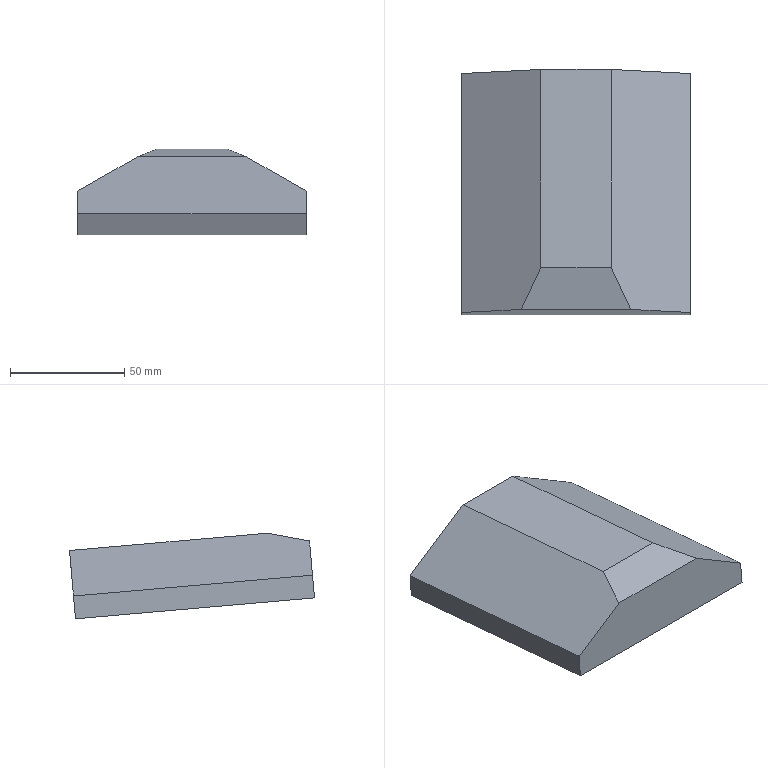Part | NX | features solid 2 | 1 solid | 9 faces | box 100 x 107.215 x 37.466 mm | volume 240609 mm3 | plane 9
STEP:
#1=CARTESIAN_POINT('',(90.,-258.715,-99.315));
#2=VERTEX_POINT('',#1);
#3=CARTESIAN_POINT('',(90.,-154.115,-108.466));
#4=VERTEX_POINT('',#3);
#5=CARTESIAN_POINT('',(90.,-258.715,-99.315));
#6=DIRECTION('',(0.,0.9962,-0.08716));
#7=VECTOR('',#6,1000.);
#8=LINE('',#5,#7);
#9=EDGE_CURVE('',#2,#4,#8,.T.);
#10=ORIENTED_EDGE('',*,*,#9,.T.);
#11=CARTESIAN_POINT('',(190.,-154.115,-108.466));
#12=VERTEX_POINT('',#11);
#13=CARTESIAN_POINT('',(190.,-154.115,-108.466));
#14=DIRECTION('',(-1.,0.,0.));
#15=VECTOR('',#14,1000.);
#16=LINE('',#13,#15);
#17=EDGE_CURVE('',#12,#4,#16,.T.);
#18=ORIENTED_EDGE('',*,*,#17,.F.);
#19=CARTESIAN_POINT('',(190.,-258.715,-99.315));
#20=VERTEX_POINT('',#19);
#21=CARTESIAN_POINT('',(190.,-258.715,-99.315));
#22=DIRECTION('',(0.,0.9962,-0.08716));
#23=VECTOR('',#22,1000.);
#24=LINE('',#21,#23);
#25=EDGE_CURVE('',#20,#12,#24,.T.);
#26=ORIENTED_EDGE('',*,*,#25,.F.);
#27=CARTESIAN_POINT('',(190.,-258.715,-99.315));
#28=DIRECTION('',(-1.,0.,0.));
#29=VECTOR('',#28,1000.);
#30=LINE('',#27,#29);
#31=EDGE_CURVE('',#20,#2,#30,.T.);
#32=ORIENTED_EDGE('',*,*,#31,.T.);
#33=EDGE_LOOP('',(#10,#18,#26,#32));
#34=FACE_BOUND('',#33,.T.);
#35=CARTESIAN_POINT('',(190.,-258.715,-99.315));
#36=DIRECTION('',(0.,0.08716,0.9962));
#37=DIRECTION('',(0.,0.9962,-0.08716));
#38=AXIS2_PLACEMENT_3D('',#35,#36,#37);
#39=PLANE('',#38);
#40=ADVANCED_FACE('',(#34),#39,.F.);
#41=CARTESIAN_POINT('',(190.,-257.844,-89.353));
#42=VERTEX_POINT('',#41);
#43=CARTESIAN_POINT('',(190.,-256.537,-74.41));
#44=DIRECTION('',(0.,-0.08716,-0.9962));
#45=VECTOR('',#44,1000.);
#46=LINE('',#43,#45);
#47=EDGE_CURVE('',#42,#20,#46,.T.);
#48=ORIENTED_EDGE('',*,*,#47,.F.);
#49=CARTESIAN_POINT('',(164.019,-256.537,-74.41));
#50=VERTEX_POINT('',#49);
#51=CARTESIAN_POINT('',(190.,-257.844,-89.353));
#52=DIRECTION('',(0.866,-0.04358,-0.4981));
#53=VECTOR('',#52,1000.);
#54=LINE('',#51,#53);
#55=EDGE_CURVE('',#42,#50,#54,.F.);
#56=ORIENTED_EDGE('',*,*,#55,.T.);
#57=CARTESIAN_POINT('',(115.981,-256.537,-74.41));
#58=VERTEX_POINT('',#57);
#59=CARTESIAN_POINT('',(190.,-256.537,-74.41));
#60=DIRECTION('',(-1.,0.,0.));
#61=VECTOR('',#60,1000.);
#62=LINE('',#59,#61);
#63=EDGE_CURVE('',#50,#58,#62,.T.);
#64=ORIENTED_EDGE('',*,*,#63,.T.);
#65=CARTESIAN_POINT('',(90.,-257.844,-89.353));
#66=VERTEX_POINT('',#65);
#67=CARTESIAN_POINT('',(124.641,-256.101,-69.429));
#68=DIRECTION('',(-0.866,-0.04358,-0.4981));
#69=VECTOR('',#68,1000.);
#70=LINE('',#67,#69);
#71=EDGE_CURVE('',#58,#66,#70,.T.);
#72=ORIENTED_EDGE('',*,*,#71,.T.);
#73=CARTESIAN_POINT('',(90.,-256.537,-74.41));
#74=DIRECTION('',(0.,-0.08716,-0.9962));
#75=VECTOR('',#74,1000.);
#76=LINE('',#73,#75);
#77=EDGE_CURVE('',#66,#2,#76,.T.);
#78=ORIENTED_EDGE('',*,*,#77,.T.);
#79=ORIENTED_EDGE('',*,*,#31,.F.);
#80=EDGE_LOOP('',(#48,#56,#64,#72,#78,#79));
#81=FACE_BOUND('',#80,.T.);
#82=CARTESIAN_POINT('',(190.,-256.537,-74.41));
#83=DIRECTION('',(0.,0.9962,-0.08716));
#84=DIRECTION('',(0.,-0.08716,-0.9962));
#85=AXIS2_PLACEMENT_3D('',#82,#83,#84);
#86=PLANE('',#85);
#87=ADVANCED_FACE('',(#81),#86,.F.);
#88=ORIENTED_EDGE('',*,*,#63,.F.);
#89=CARTESIAN_POINT('',(155.359,-238.141,-71.));
#90=VERTEX_POINT('',#89);
#91=CARTESIAN_POINT('',(152.571,-232.219,-69.902));
#92=DIRECTION('',(0.4201,-0.8923,-0.1654));
#93=VECTOR('',#92,1000.);
#94=LINE('',#91,#93);
#95=EDGE_CURVE('',#50,#90,#94,.F.);
#96=ORIENTED_EDGE('',*,*,#95,.T.);
#97=CARTESIAN_POINT('',(124.641,-238.141,-71.));
#98=VERTEX_POINT('',#97);
#99=CARTESIAN_POINT('',(190.,-238.141,-71.));
#100=DIRECTION('',(-1.,0.,0.));
#101=VECTOR('',#100,1000.);
#102=LINE('',#99,#101);
#103=EDGE_CURVE('',#90,#98,#102,.T.);
#104=ORIENTED_EDGE('',*,*,#103,.T.);
#105=CARTESIAN_POINT('',(164.672,-153.112,-55.239));
#106=DIRECTION('',(-0.4201,-0.8923,-0.1654));
#107=VECTOR('',#106,1000.);
#108=LINE('',#105,#107);
#109=EDGE_CURVE('',#98,#58,#108,.T.);
#110=ORIENTED_EDGE('',*,*,#109,.T.);
#111=EDGE_LOOP('',(#88,#96,#104,#110));
#112=FACE_BOUND('',#111,.T.);
#113=CARTESIAN_POINT('',(190.,-238.141,-71.));
#114=DIRECTION('',(0.,0.1823,-0.9833));
#115=DIRECTION('',(0.,-0.9833,-0.1823));
#116=AXIS2_PLACEMENT_3D('',#113,#114,#115);
#117=PLANE('',#116);
#118=ADVANCED_FACE('',(#112),#117,.F.);
#119=ORIENTED_EDGE('',*,*,#103,.F.);
#120=CARTESIAN_POINT('',(155.359,-151.5,-78.58));
#121=VERTEX_POINT('',#120);
#122=CARTESIAN_POINT('',(155.359,-129.584,-80.498));
#123=DIRECTION('',(0.,0.9962,-0.08716));
#124=VECTOR('',#123,1000.);
#125=LINE('',#122,#124);
#126=EDGE_CURVE('',#90,#121,#125,.T.);
#127=ORIENTED_EDGE('',*,*,#126,.T.);
#128=CARTESIAN_POINT('',(124.641,-151.5,-78.58));
#129=VERTEX_POINT('',#128);
#130=CARTESIAN_POINT('',(190.,-151.5,-78.58));
#131=DIRECTION('',(-1.,0.,0.));
#132=VECTOR('',#131,1000.);
#133=LINE('',#130,#132);
#134=EDGE_CURVE('',#121,#129,#133,.T.);
#135=ORIENTED_EDGE('',*,*,#134,.T.);
#136=CARTESIAN_POINT('',(124.641,-238.141,-71.));
#137=DIRECTION('',(0.,-0.9962,0.08716));
#138=VECTOR('',#137,1000.);
#139=LINE('',#136,#138);
#140=EDGE_CURVE('',#129,#98,#139,.T.);
#141=ORIENTED_EDGE('',*,*,#140,.T.);
#142=EDGE_LOOP('',(#119,#127,#135,#141));
#143=FACE_BOUND('',#142,.T.);
#144=CARTESIAN_POINT('',(190.,-129.584,-80.498));
#145=DIRECTION('',(0.,-0.08716,-0.9962));
#146=DIRECTION('',(0.,-0.9962,0.08716));
#147=AXIS2_PLACEMENT_3D('',#144,#145,#146);
#148=PLANE('',#147);
#149=ADVANCED_FACE('',(#143),#148,.F.);
#150=ORIENTED_EDGE('',*,*,#134,.F.);
#151=CARTESIAN_POINT('',(190.,-153.243,-98.504));
#152=VERTEX_POINT('',#151);
#153=CARTESIAN_POINT('',(181.34,-152.808,-93.523));
#154=DIRECTION('',(-0.866,0.04358,0.4981));
#155=VECTOR('',#154,1000.);
#156=LINE('',#153,#155);
#157=EDGE_CURVE('',#121,#152,#156,.F.);
#158=ORIENTED_EDGE('',*,*,#157,.T.);
#159=CARTESIAN_POINT('',(190.,-151.5,-78.58));
#160=DIRECTION('',(0.,-0.08716,-0.9962));
#161=VECTOR('',#160,1000.);
#162=LINE('',#159,#161);
#163=EDGE_CURVE('',#152,#12,#162,.T.);
#164=ORIENTED_EDGE('',*,*,#163,.T.);
#165=ORIENTED_EDGE('',*,*,#17,.T.);
#166=CARTESIAN_POINT('',(90.,-153.243,-98.504));
#167=VERTEX_POINT('',#166);
#168=CARTESIAN_POINT('',(90.,-151.5,-78.58));
#169=DIRECTION('',(0.,-0.08716,-0.9962));
#170=VECTOR('',#169,1000.);
#171=LINE('',#168,#170);
#172=EDGE_CURVE('',#167,#4,#171,.T.);
#173=ORIENTED_EDGE('',*,*,#172,.F.);
#174=CARTESIAN_POINT('',(173.66,-149.034,-50.387));
#175=DIRECTION('',(0.866,0.04358,0.4981));
#176=VECTOR('',#175,1000.);
#177=LINE('',#174,#176);
#178=EDGE_CURVE('',#167,#129,#177,.T.);
#179=ORIENTED_EDGE('',*,*,#178,.T.);
#180=EDGE_LOOP('',(#150,#158,#164,#165,#173,#179));
#181=FACE_BOUND('',#180,.T.);
#182=CARTESIAN_POINT('',(190.,-151.5,-78.58));
#183=DIRECTION('',(0.,0.9962,-0.08716));
#184=DIRECTION('',(0.,-0.08716,-0.9962));
#185=AXIS2_PLACEMENT_3D('',#182,#183,#184);
#186=PLANE('',#185);
#187=ADVANCED_FACE('',(#181),#186,.T.);
#188=ORIENTED_EDGE('',*,*,#163,.F.);
#189=CARTESIAN_POINT('',(190.,-210.22,-93.519));
#190=DIRECTION('',(0.,-0.9962,0.08716));
#191=VECTOR('',#190,1000.);
#192=LINE('',#189,#191);
#193=EDGE_CURVE('',#152,#42,#192,.T.);
#194=ORIENTED_EDGE('',*,*,#193,.T.);
#195=ORIENTED_EDGE('',*,*,#47,.T.);
#196=ORIENTED_EDGE('',*,*,#25,.T.);
#197=EDGE_LOOP('',(#188,#194,#195,#196));
#198=FACE_BOUND('',#197,.T.);
#199=CARTESIAN_POINT('',(190.,-209.61,-86.546));
#200=DIRECTION('',(-1.,0.,0.));
#201=DIRECTION('',(0.,0.,1.));
#202=AXIS2_PLACEMENT_3D('',#199,#200,#201);
#203=PLANE('',#202);
#204=ADVANCED_FACE('',(#198),#203,.F.);
#205=ORIENTED_EDGE('',*,*,#77,.F.);
#206=CARTESIAN_POINT('',(90.,-153.243,-98.504));
#207=DIRECTION('',(0.,0.9962,-0.08716));
#208=VECTOR('',#207,1000.);
#209=LINE('',#206,#208);
#210=EDGE_CURVE('',#66,#167,#209,.T.);
#211=ORIENTED_EDGE('',*,*,#210,.T.);
#212=ORIENTED_EDGE('',*,*,#172,.T.);
#213=ORIENTED_EDGE('',*,*,#9,.F.);
#214=EDGE_LOOP('',(#205,#211,#212,#213));
#215=FACE_BOUND('',#214,.T.);
#216=CARTESIAN_POINT('',(90.,-209.61,-86.546));
#217=DIRECTION('',(-1.,0.,0.));
#218=DIRECTION('',(0.,0.,1.));
#219=AXIS2_PLACEMENT_3D('',#216,#217,#218);
#220=PLANE('',#219);
#221=ADVANCED_FACE('',(#215),#220,.T.);
#222=ORIENTED_EDGE('',*,*,#178,.F.);
#223=ORIENTED_EDGE('',*,*,#210,.F.);
#224=ORIENTED_EDGE('',*,*,#71,.F.);
#225=ORIENTED_EDGE('',*,*,#109,.F.);
#226=ORIENTED_EDGE('',*,*,#140,.F.);
#227=EDGE_LOOP('',(#222,#223,#224,#225,#226));
#228=FACE_BOUND('',#227,.T.);
#229=CARTESIAN_POINT('',(124.641,-129.584,-80.498));
#230=DIRECTION('',(-0.5,0.07548,0.8627));
#231=DIRECTION('',(0.8652,0.,0.5014));
#232=AXIS2_PLACEMENT_3D('',#229,#230,#231);
#233=PLANE('',#232);
#234=ADVANCED_FACE('',(#228),#233,.T.);
#235=ORIENTED_EDGE('',*,*,#157,.F.);
#236=ORIENTED_EDGE('',*,*,#126,.F.);
#237=ORIENTED_EDGE('',*,*,#95,.F.);
#238=ORIENTED_EDGE('',*,*,#55,.F.);
#239=ORIENTED_EDGE('',*,*,#193,.F.);
#240=EDGE_LOOP('',(#235,#236,#237,#238,#239));
#241=FACE_BOUND('',#240,.T.);
#242=CARTESIAN_POINT('',(190.,-210.22,-93.519));
#243=DIRECTION('',(-0.5,-0.07548,-0.8627));
#244=DIRECTION('',(-0.8652,0.,0.5014));
#245=AXIS2_PLACEMENT_3D('',#242,#243,#244);
#246=PLANE('',#245);
#247=ADVANCED_FACE('',(#241),#246,.F.);
#248=CLOSED_SHELL('',(#40,#87,#118,#149,#187,#204,#221,#234,#247));
#249=MANIFOLD_SOLID_BREP('',#248);
#250=(LENGTH_UNIT()NAMED_UNIT(*)SI_UNIT(.MILLI.,.METRE.));
#251=UNCERTAINTY_MEASURE_WITH_UNIT(LENGTH_MEASURE(0.00001),#250,'','');
#252=(NAMED_UNIT(*)PLANE_ANGLE_UNIT()SI_UNIT($,.RADIAN.));
#253=(NAMED_UNIT(*)SI_UNIT($,.STERADIAN.)SOLID_ANGLE_UNIT());
#254=(GEOMETRIC_REPRESENTATION_CONTEXT(3)GLOBAL_UNCERTAINTY_ASSIGNED_CONTEXT((#251))GLOBAL_UNIT_ASSIGNED_CONTEXT((#250,#252,#253))REPRESENTATION_CONTEXT('',''));
#255=ADVANCED_BREP_SHAPE_REPRESENTATION('',(#249),#254);